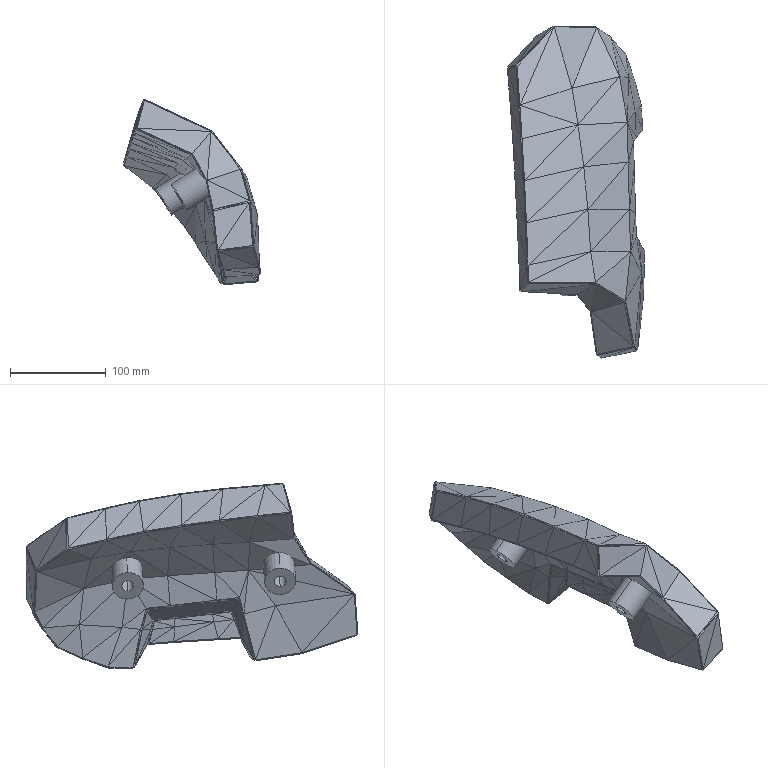Part | SolidWorks | features MirrorStock 1 | 1 solid | 429 faces | box 143.42 x 346.686 x 193.978 mm | volume 2031245 mm3 | plane 421 | cylinder 8 | commonest cylinder face diameters 12.5 x4 32.5 x4